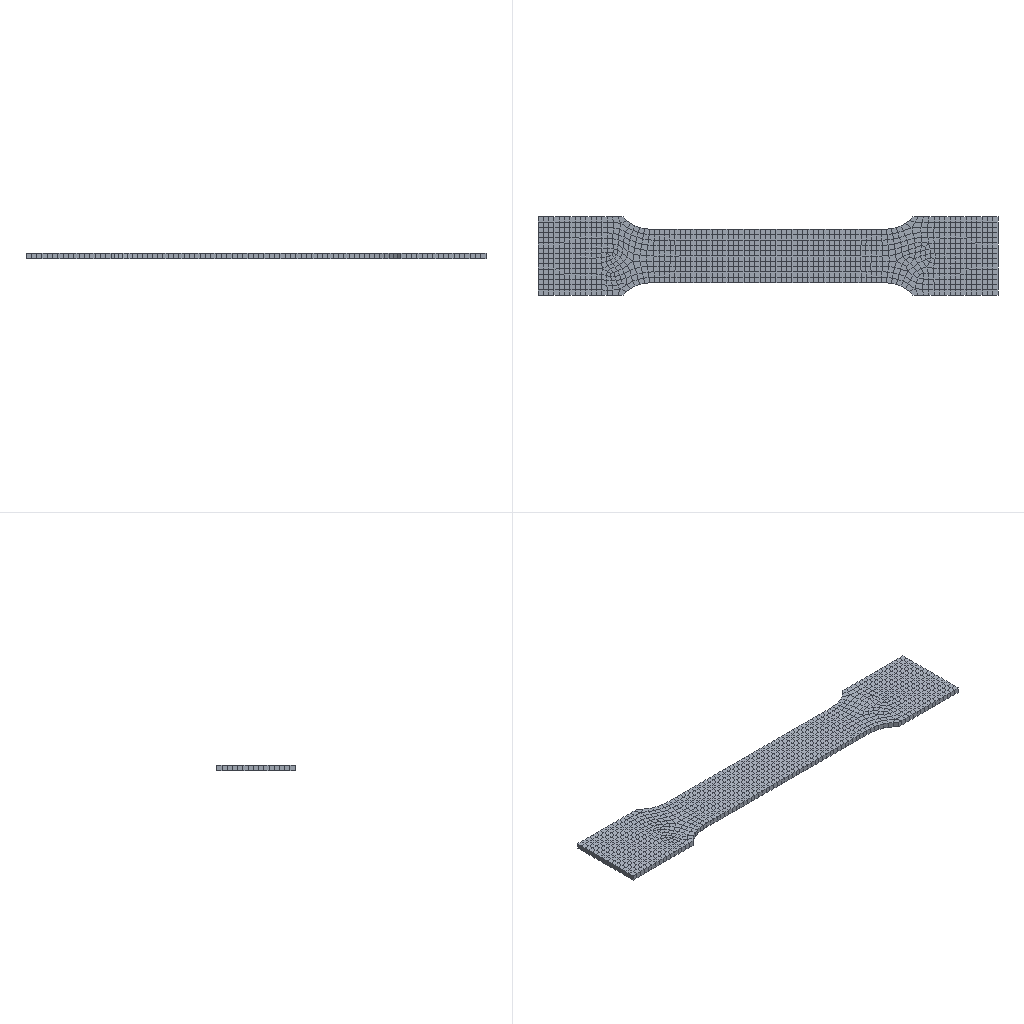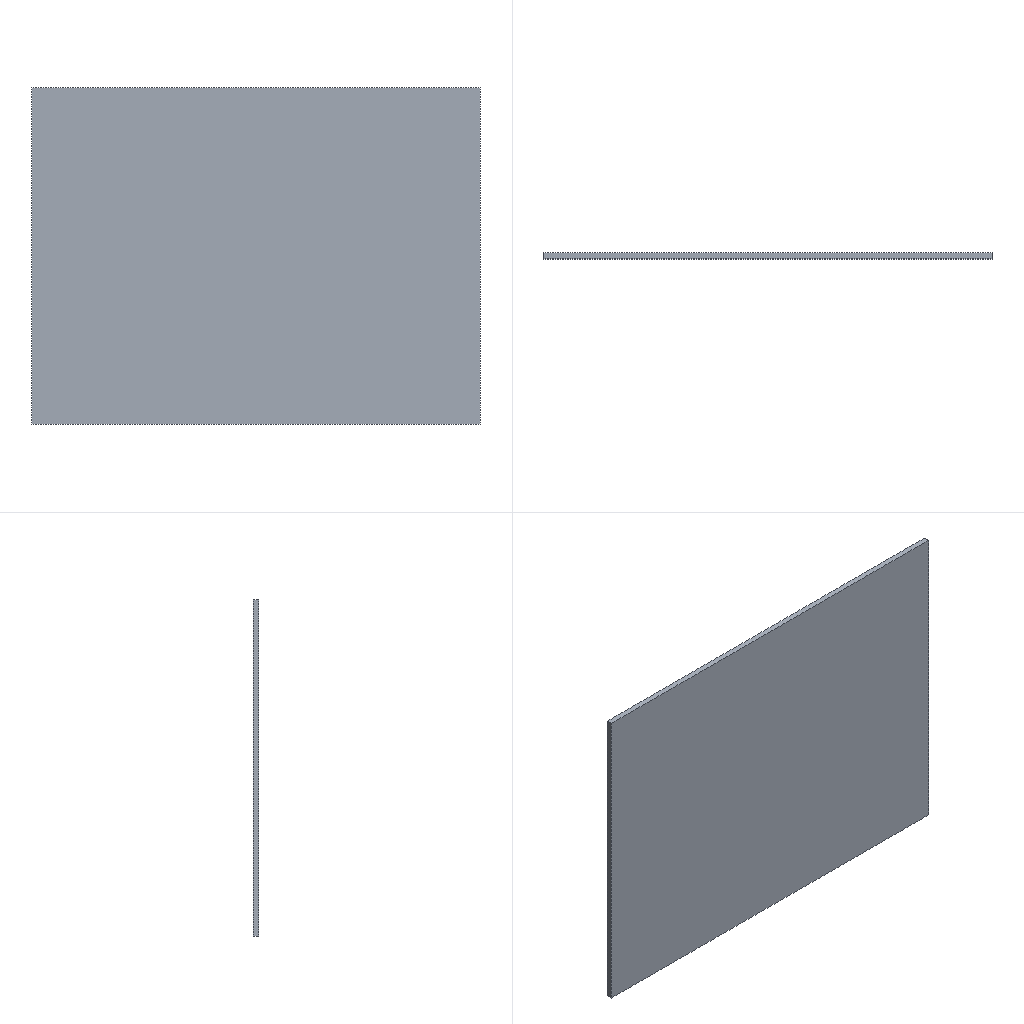Simulation study | ansys workbench
Set-up summary:
category,name,step,type,value,unit,region
solver,ansys_mapdl
solver,version,,,22.1
solver,version,,,22.1
units,MPA,,stated
analysis,deck1,,static,static
load_step,requested,,,1
analysis,nlgeom,,,False
mesh,nodes,,,1021147
mesh,elements,,,217336
element_type,ANSYS 186 (type 1),,solid,213600
element_type,ANSYS 154 (type 2),,surface,1068
element_type,ANSYS 154 (type 3),,surface,1068
element_type,ANSYS 154 (type 4),,surface,800
element_type,ANSYS 154 (type 5),,surface,800
load,load commands in deck,,count,12
bc,support commands in deck,,count,3
named_set,_DISPZEROUX,,component
named_set,_DISPZEROUY,,component
named_set,_DISPZEROUZ,,component
analysis,deck2,,static,static
load_step,requested,,,1
analysis,nlgeom,,,False
mesh,nodes,,,7714
mesh,elements,,,1043
element_type,ANSYS 186 (type 1),,solid,1028
element_type,ANSYS 154 (type 2),,surface,15
load,load commands in deck,,count,3
bc,support commands in deck,,count,3
named_set,_DISPZEROUX,,component
named_set,_DISPZEROUY,,component
named_set,_DISPZEROUZ,,component
material,1,,in results
material,1,,in results
check,setup vs results,,match,3736 surface effect element(s) are not in the reader's mesh and were not compared
check,setup vs results,,match,15 surface effect element(s) are not in the reader's mesh and were not compared
Results summary:
result,analysis,,,static
result,last_loadstep,,,1
result,primary field,,,displacement
result,reaction total,1,FX,-0.0,N
result,reaction total,1,FY,0.0,N
result,reaction total,1,FZ,0.0,N
result,mass,,,0.03768,"NMM: mm, ton, N, s, mV, mA, degC"
result,analysis,,,static
result,last_loadstep,,,1
result,primary field,,,displacement
result,reaction total,1,FX,-6000,N
result,reaction total,1,FY,0.0,N
result,reaction total,1,FZ,0.0,N
result,mass,,,6.5e-05,"NMM: mm, ton, N, s, mV, mA, degC"